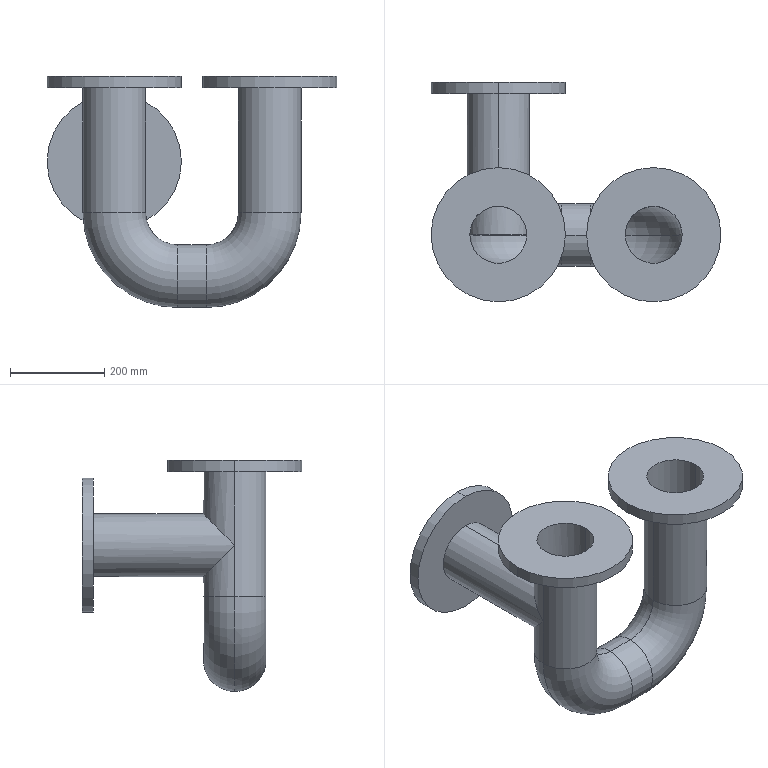Part | SolidWorks | features ICE 3, Sweep 1 | 1 solid | 48 faces | box 615 x 466.5 x 490.5 mm | volume 6883976 mm3 | cylinder 32 | torus 8 | plane 8 | commonest cylinder face diameters 121 x13 133 x13 285 x6